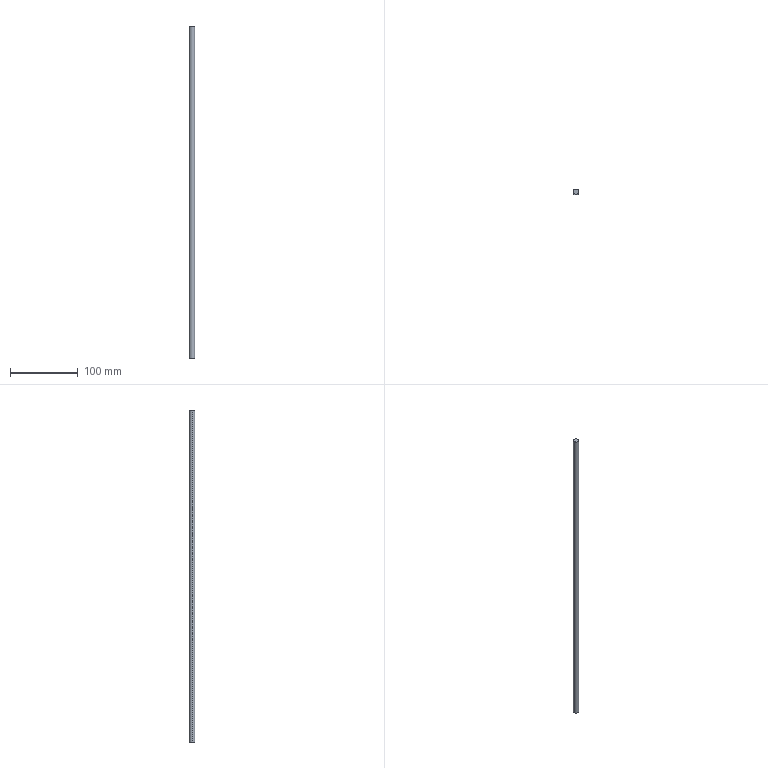Part | STEP file | Sprocket 1 shaft | 1 solid | 4 faces | box 8 x 8 x 490 mm | volume 24630 mm3 | cylinder 2 | plane 2 | commonest cylinder face diameters 8 x2
STEP:
#1=CARTESIAN_POINT('',(0.,0.,0.));
#2=DIRECTION('',(0.,0.,1.));
#3=DIRECTION('',(1.,0.,0.));
#4=AXIS2_PLACEMENT_3D('',#1,#2,#3);
#5=CARTESIAN_POINT('',(4.,0.,490.));
#6=VERTEX_POINT('',#5);
#7=CARTESIAN_POINT('',(-4.,0.,490.));
#8=VERTEX_POINT('',#7);
#9=CARTESIAN_POINT('',(0.,0.,490.));
#10=DIRECTION('',(0.,0.,1.));
#11=DIRECTION('',(1.,0.,0.));
#12=AXIS2_PLACEMENT_3D('',#9,#10,#11);
#13=CIRCLE('',#12,4.);
#14=CARTESIAN_POINT('',(0.,0.,490.));
#15=DIRECTION('',(0.,0.,-1.));
#16=DIRECTION('',(-1.,0.,0.));
#17=AXIS2_PLACEMENT_3D('',#14,#15,#16);
#18=CYLINDRICAL_SURFACE('',#17,4.);
#19=CARTESIAN_POINT('',(3.142,0.));
#20=DIRECTION('',(-1.,0.));
#21=VECTOR('',#20,1.);
#22=LINE('',#19,#21);
#23=(GEOMETRIC_REPRESENTATION_CONTEXT(2)PARAMETRIC_REPRESENTATION_CONTEXT()REPRESENTATION_CONTEXT('',''));
#24=DEFINITIONAL_REPRESENTATION('',(#22),#23);
#25=PCURVE('',#18,#24);
#26=CARTESIAN_POINT('',(0.,0.,490.));
#27=DIRECTION('',(0.,0.,1.));
#28=DIRECTION('',(1.,0.,0.));
#29=AXIS2_PLACEMENT_3D('',#26,#27,#28);
#30=PLANE('',#29);
#31=CARTESIAN_POINT('',(0.,0.));
#32=DIRECTION('',(1.,0.));
#33=AXIS2_PLACEMENT_2D('',#31,#32);
#34=CIRCLE('',#33,4.);
#35=(GEOMETRIC_REPRESENTATION_CONTEXT(2)PARAMETRIC_REPRESENTATION_CONTEXT()REPRESENTATION_CONTEXT('',''));
#36=DEFINITIONAL_REPRESENTATION('',(#34),#35);
#37=PCURVE('',#30,#36);
#38=SURFACE_CURVE('',#13,(#25,#37),.PCURVE_S1.);
#39=EDGE_CURVE('',#6,#8,#38,.T.);
#40=ORIENTED_EDGE('',*,*,#39,.F.);
#41=CARTESIAN_POINT('',(4.,0.,0.));
#42=VERTEX_POINT('',#41);
#43=CARTESIAN_POINT('',(4.,0.,490.));
#44=DIRECTION('',(0.,0.,-1.));
#45=VECTOR('',#44,1.);
#46=LINE('',#43,#45);
#47=CARTESIAN_POINT('',(3.142,0.));
#48=DIRECTION('',(0.,1.));
#49=VECTOR('',#48,1.);
#50=LINE('',#47,#49);
#51=(GEOMETRIC_REPRESENTATION_CONTEXT(2)PARAMETRIC_REPRESENTATION_CONTEXT()REPRESENTATION_CONTEXT('',''));
#52=DEFINITIONAL_REPRESENTATION('',(#50),#51);
#53=PCURVE('',#18,#52);
#54=CARTESIAN_POINT('',(0.,0.,490.));
#55=DIRECTION('',(0.,0.,-1.));
#56=DIRECTION('',(-1.,0.,0.));
#57=AXIS2_PLACEMENT_3D('',#54,#55,#56);
#58=CYLINDRICAL_SURFACE('',#57,4.);
#59=CARTESIAN_POINT('',(3.142,0.));
#60=DIRECTION('',(0.,1.));
#61=VECTOR('',#60,1.);
#62=LINE('',#59,#61);
#63=(GEOMETRIC_REPRESENTATION_CONTEXT(2)PARAMETRIC_REPRESENTATION_CONTEXT()REPRESENTATION_CONTEXT('',''));
#64=DEFINITIONAL_REPRESENTATION('',(#62),#63);
#65=PCURVE('',#58,#64);
#66=SURFACE_CURVE('',#46,(#53,#65),.PCURVE_S1.);
#67=EDGE_CURVE('',#6,#42,#66,.T.);
#68=ORIENTED_EDGE('',*,*,#67,.T.);
#69=CARTESIAN_POINT('',(-4.,0.,0.));
#70=VERTEX_POINT('',#69);
#71=CARTESIAN_POINT('',(0.,0.,0.));
#72=DIRECTION('',(0.,0.,1.));
#73=DIRECTION('',(1.,0.,0.));
#74=AXIS2_PLACEMENT_3D('',#71,#72,#73);
#75=CIRCLE('',#74,4.);
#76=CARTESIAN_POINT('',(3.142,490.));
#77=DIRECTION('',(-1.,0.));
#78=VECTOR('',#77,1.);
#79=LINE('',#76,#78);
#80=(GEOMETRIC_REPRESENTATION_CONTEXT(2)PARAMETRIC_REPRESENTATION_CONTEXT()REPRESENTATION_CONTEXT('',''));
#81=DEFINITIONAL_REPRESENTATION('',(#79),#80);
#82=PCURVE('',#18,#81);
#83=CARTESIAN_POINT('',(0.,0.,0.));
#84=DIRECTION('',(0.,0.,1.));
#85=DIRECTION('',(1.,0.,0.));
#86=AXIS2_PLACEMENT_3D('',#83,#84,#85);
#87=PLANE('',#86);
#88=CARTESIAN_POINT('',(0.,0.));
#89=DIRECTION('',(1.,0.));
#90=AXIS2_PLACEMENT_2D('',#88,#89);
#91=CIRCLE('',#90,4.);
#92=(GEOMETRIC_REPRESENTATION_CONTEXT(2)PARAMETRIC_REPRESENTATION_CONTEXT()REPRESENTATION_CONTEXT('',''));
#93=DEFINITIONAL_REPRESENTATION('',(#91),#92);
#94=PCURVE('',#87,#93);
#95=SURFACE_CURVE('',#75,(#82,#94),.PCURVE_S1.);
#96=EDGE_CURVE('',#42,#70,#95,.T.);
#97=ORIENTED_EDGE('',*,*,#96,.T.);
#98=CARTESIAN_POINT('',(-4.,0.,490.));
#99=DIRECTION('',(0.,0.,-1.));
#100=VECTOR('',#99,1.);
#101=LINE('',#98,#100);
#102=CARTESIAN_POINT('',(0.,0.));
#103=DIRECTION('',(0.,1.));
#104=VECTOR('',#103,1.);
#105=LINE('',#102,#104);
#106=(GEOMETRIC_REPRESENTATION_CONTEXT(2)PARAMETRIC_REPRESENTATION_CONTEXT()REPRESENTATION_CONTEXT('',''));
#107=DEFINITIONAL_REPRESENTATION('',(#105),#106);
#108=PCURVE('',#18,#107);
#109=CARTESIAN_POINT('',(6.283,0.));
#110=DIRECTION('',(0.,1.));
#111=VECTOR('',#110,1.);
#112=LINE('',#109,#111);
#113=(GEOMETRIC_REPRESENTATION_CONTEXT(2)PARAMETRIC_REPRESENTATION_CONTEXT()REPRESENTATION_CONTEXT('',''));
#114=DEFINITIONAL_REPRESENTATION('',(#112),#113);
#115=PCURVE('',#58,#114);
#116=SURFACE_CURVE('',#101,(#108,#115),.PCURVE_S1.);
#117=EDGE_CURVE('',#8,#70,#116,.T.);
#118=ORIENTED_EDGE('',*,*,#117,.F.);
#119=EDGE_LOOP('',(#40,#68,#97,#118));
#120=FACE_BOUND('',#119,.T.);
#121=ADVANCED_FACE('',(#120),#18,.T.);
#122=ORIENTED_EDGE('',*,*,#67,.F.);
#123=CARTESIAN_POINT('',(0.,0.,490.));
#124=DIRECTION('',(0.,0.,1.));
#125=DIRECTION('',(1.,0.,0.));
#126=AXIS2_PLACEMENT_3D('',#123,#124,#125);
#127=CIRCLE('',#126,4.);
#128=CARTESIAN_POINT('',(9.425,0.));
#129=DIRECTION('',(-1.,0.));
#130=VECTOR('',#129,1.);
#131=LINE('',#128,#130);
#132=(GEOMETRIC_REPRESENTATION_CONTEXT(2)PARAMETRIC_REPRESENTATION_CONTEXT()REPRESENTATION_CONTEXT('',''));
#133=DEFINITIONAL_REPRESENTATION('',(#131),#132);
#134=PCURVE('',#58,#133);
#135=CARTESIAN_POINT('',(0.,0.));
#136=DIRECTION('',(1.,0.));
#137=AXIS2_PLACEMENT_2D('',#135,#136);
#138=CIRCLE('',#137,4.);
#139=(GEOMETRIC_REPRESENTATION_CONTEXT(2)PARAMETRIC_REPRESENTATION_CONTEXT()REPRESENTATION_CONTEXT('',''));
#140=DEFINITIONAL_REPRESENTATION('',(#138),#139);
#141=PCURVE('',#30,#140);
#142=SURFACE_CURVE('',#127,(#134,#141),.PCURVE_S1.);
#143=EDGE_CURVE('',#8,#6,#142,.T.);
#144=ORIENTED_EDGE('',*,*,#143,.F.);
#145=ORIENTED_EDGE('',*,*,#117,.T.);
#146=CARTESIAN_POINT('',(0.,0.,0.));
#147=DIRECTION('',(0.,0.,1.));
#148=DIRECTION('',(1.,0.,0.));
#149=AXIS2_PLACEMENT_3D('',#146,#147,#148);
#150=CIRCLE('',#149,4.);
#151=CARTESIAN_POINT('',(9.425,490.));
#152=DIRECTION('',(-1.,0.));
#153=VECTOR('',#152,1.);
#154=LINE('',#151,#153);
#155=(GEOMETRIC_REPRESENTATION_CONTEXT(2)PARAMETRIC_REPRESENTATION_CONTEXT()REPRESENTATION_CONTEXT('',''));
#156=DEFINITIONAL_REPRESENTATION('',(#154),#155);
#157=PCURVE('',#58,#156);
#158=CARTESIAN_POINT('',(0.,0.));
#159=DIRECTION('',(1.,0.));
#160=AXIS2_PLACEMENT_2D('',#158,#159);
#161=CIRCLE('',#160,4.);
#162=(GEOMETRIC_REPRESENTATION_CONTEXT(2)PARAMETRIC_REPRESENTATION_CONTEXT()REPRESENTATION_CONTEXT('',''));
#163=DEFINITIONAL_REPRESENTATION('',(#161),#162);
#164=PCURVE('',#87,#163);
#165=SURFACE_CURVE('',#150,(#157,#164),.PCURVE_S1.);
#166=EDGE_CURVE('',#70,#42,#165,.T.);
#167=ORIENTED_EDGE('',*,*,#166,.T.);
#168=EDGE_LOOP('',(#122,#144,#145,#167));
#169=FACE_BOUND('',#168,.T.);
#170=ADVANCED_FACE('',(#169),#58,.T.);
#171=ORIENTED_EDGE('',*,*,#143,.T.);
#172=ORIENTED_EDGE('',*,*,#39,.T.);
#173=EDGE_LOOP('',(#171,#172));
#174=FACE_BOUND('',#173,.T.);
#175=ADVANCED_FACE('',(#174),#30,.T.);
#176=ORIENTED_EDGE('',*,*,#166,.F.);
#177=ORIENTED_EDGE('',*,*,#96,.F.);
#178=EDGE_LOOP('',(#176,#177));
#179=FACE_BOUND('',#178,.T.);
#180=ADVANCED_FACE('',(#179),#87,.F.);
#181=CLOSED_SHELL('',(#121,#170,#175,#180));
#182=MANIFOLD_SOLID_BREP('',#181);
#183=(LENGTH_UNIT()NAMED_UNIT(*)SI_UNIT(.MILLI.,.METRE.));
#184=UNCERTAINTY_MEASURE_WITH_UNIT(LENGTH_MEASURE(0.0000001),#183,'','');
#185=(NAMED_UNIT(*)PLANE_ANGLE_UNIT()SI_UNIT($,.RADIAN.));
#186=(NAMED_UNIT(*)SI_UNIT($,.STERADIAN.)SOLID_ANGLE_UNIT());
#187=(GEOMETRIC_REPRESENTATION_CONTEXT(3)GLOBAL_UNCERTAINTY_ASSIGNED_CONTEXT((#184))GLOBAL_UNIT_ASSIGNED_CONTEXT((#183,#185,#186))REPRESENTATION_CONTEXT('',''));
#188=ADVANCED_BREP_SHAPE_REPRESENTATION('',(#4,#182),#187);